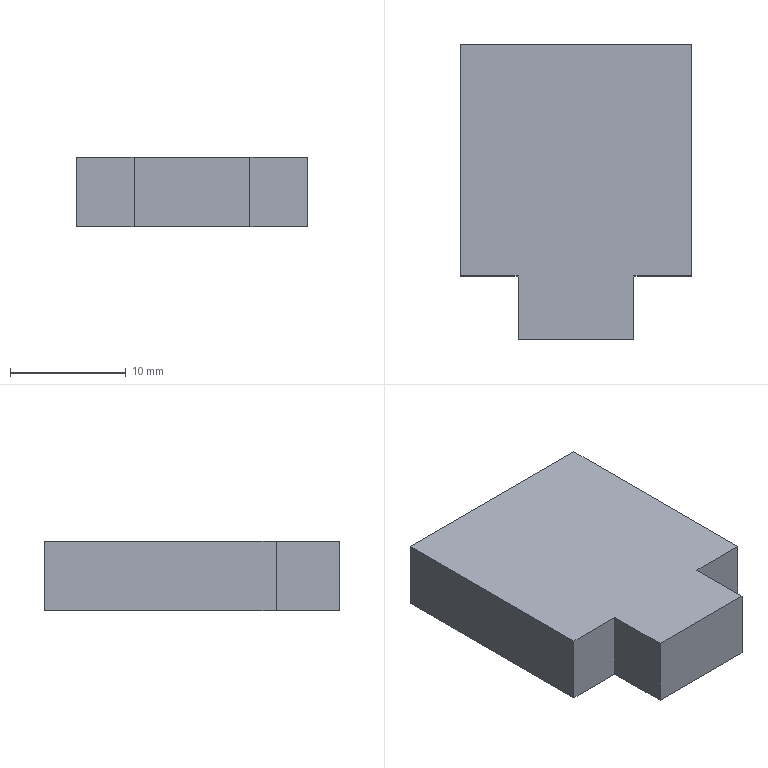Part | SolidWorks | features FlatPattern 1, SMBaseFlange 1, SheetMetal 1 | 1 solid | 10 faces | box 20 x 25.5 x 6 mm | volume 2730 mm3 | plane 10
STEP:
#1=CARTESIAN_POINT('',(50.677,0.,0.));
#2=VERTEX_POINT('',#1);
#3=CARTESIAN_POINT('',(50.677,-5.5,0.));
#4=VERTEX_POINT('',#3);
#5=CARTESIAN_POINT('',(50.677,0.,0.));
#6=DIRECTION('',(0.,-1.,0.));
#7=VECTOR('',#6,1000.);
#8=LINE('',#5,#7);
#9=EDGE_CURVE('',#2,#4,#8,.T.);
#10=ORIENTED_EDGE('',*,*,#9,.T.);
#11=CARTESIAN_POINT('',(50.677,-5.5,6.));
#12=VERTEX_POINT('',#11);
#13=CARTESIAN_POINT('',(50.677,-5.5,6.));
#14=DIRECTION('',(0.,0.,-1.));
#15=VECTOR('',#14,1000.);
#16=LINE('',#13,#15);
#17=EDGE_CURVE('',#12,#4,#16,.T.);
#18=ORIENTED_EDGE('',*,*,#17,.F.);
#19=CARTESIAN_POINT('',(50.677,0.,6.));
#20=VERTEX_POINT('',#19);
#21=CARTESIAN_POINT('',(50.677,0.,6.));
#22=DIRECTION('',(0.,-1.,0.));
#23=VECTOR('',#22,1000.);
#24=LINE('',#21,#23);
#25=EDGE_CURVE('',#20,#12,#24,.T.);
#26=ORIENTED_EDGE('',*,*,#25,.F.);
#27=CARTESIAN_POINT('',(50.677,0.,6.));
#28=DIRECTION('',(0.,0.,-1.));
#29=VECTOR('',#28,1000.);
#30=LINE('',#27,#29);
#31=EDGE_CURVE('',#20,#2,#30,.T.);
#32=ORIENTED_EDGE('',*,*,#31,.T.);
#33=EDGE_LOOP('',(#10,#18,#26,#32));
#34=FACE_OUTER_BOUND('',#33,.T.);
#35=CARTESIAN_POINT('',(50.677,0.,6.));
#36=DIRECTION('',(1.,0.,0.));
#37=DIRECTION('',(0.,0.,-1.));
#38=AXIS2_PLACEMENT_3D('',#35,#36,#37);
#39=PLANE('',#38);
#40=ADVANCED_FACE('',(#34),#39,.F.);
#41=CARTESIAN_POINT('',(60.677,-5.5,0.));
#42=VERTEX_POINT('',#41);
#43=CARTESIAN_POINT('',(50.677,-5.5,0.));
#44=DIRECTION('',(1.,0.,0.));
#45=VECTOR('',#44,1000.);
#46=LINE('',#43,#45);
#47=EDGE_CURVE('',#4,#42,#46,.T.);
#48=ORIENTED_EDGE('',*,*,#47,.T.);
#49=CARTESIAN_POINT('',(60.677,-5.5,6.));
#50=VERTEX_POINT('',#49);
#51=CARTESIAN_POINT('',(60.677,-5.5,6.));
#52=DIRECTION('',(0.,0.,-1.));
#53=VECTOR('',#52,1000.);
#54=LINE('',#51,#53);
#55=EDGE_CURVE('',#50,#42,#54,.T.);
#56=ORIENTED_EDGE('',*,*,#55,.F.);
#57=CARTESIAN_POINT('',(50.677,-5.5,6.));
#58=DIRECTION('',(1.,0.,0.));
#59=VECTOR('',#58,1000.);
#60=LINE('',#57,#59);
#61=EDGE_CURVE('',#12,#50,#60,.T.);
#62=ORIENTED_EDGE('',*,*,#61,.F.);
#63=ORIENTED_EDGE('',*,*,#17,.T.);
#64=EDGE_LOOP('',(#48,#56,#62,#63));
#65=FACE_OUTER_BOUND('',#64,.T.);
#66=CARTESIAN_POINT('',(50.677,-5.5,6.));
#67=DIRECTION('',(0.,1.,0.));
#68=DIRECTION('',(0.,0.,1.));
#69=AXIS2_PLACEMENT_3D('',#66,#67,#68);
#70=PLANE('',#69);
#71=ADVANCED_FACE('',(#65),#70,.F.);
#72=CARTESIAN_POINT('',(60.677,0.,0.));
#73=VERTEX_POINT('',#72);
#74=CARTESIAN_POINT('',(60.677,-5.5,0.));
#75=DIRECTION('',(0.,1.,0.));
#76=VECTOR('',#75,1000.);
#77=LINE('',#74,#76);
#78=EDGE_CURVE('',#42,#73,#77,.T.);
#79=ORIENTED_EDGE('',*,*,#78,.T.);
#80=CARTESIAN_POINT('',(60.677,0.,6.));
#81=VERTEX_POINT('',#80);
#82=CARTESIAN_POINT('',(60.677,0.,6.));
#83=DIRECTION('',(0.,0.,-1.));
#84=VECTOR('',#83,1000.);
#85=LINE('',#82,#84);
#86=EDGE_CURVE('',#81,#73,#85,.T.);
#87=ORIENTED_EDGE('',*,*,#86,.F.);
#88=CARTESIAN_POINT('',(60.677,-5.5,6.));
#89=DIRECTION('',(0.,1.,0.));
#90=VECTOR('',#89,1000.);
#91=LINE('',#88,#90);
#92=EDGE_CURVE('',#50,#81,#91,.T.);
#93=ORIENTED_EDGE('',*,*,#92,.F.);
#94=ORIENTED_EDGE('',*,*,#55,.T.);
#95=EDGE_LOOP('',(#79,#87,#93,#94));
#96=FACE_OUTER_BOUND('',#95,.T.);
#97=CARTESIAN_POINT('',(60.677,-5.5,6.));
#98=DIRECTION('',(-1.,0.,0.));
#99=DIRECTION('',(0.,0.,1.));
#100=AXIS2_PLACEMENT_3D('',#97,#98,#99);
#101=PLANE('',#100);
#102=ADVANCED_FACE('',(#96),#101,.F.);
#103=CARTESIAN_POINT('',(65.677,0.,0.));
#104=VERTEX_POINT('',#103);
#105=CARTESIAN_POINT('',(60.677,0.,0.));
#106=DIRECTION('',(1.,0.,0.));
#107=VECTOR('',#106,1000.);
#108=LINE('',#105,#107);
#109=EDGE_CURVE('',#73,#104,#108,.T.);
#110=ORIENTED_EDGE('',*,*,#109,.T.);
#111=CARTESIAN_POINT('',(65.677,0.,6.));
#112=VERTEX_POINT('',#111);
#113=CARTESIAN_POINT('',(65.677,0.,6.));
#114=DIRECTION('',(0.,0.,-1.));
#115=VECTOR('',#114,1000.);
#116=LINE('',#113,#115);
#117=EDGE_CURVE('',#112,#104,#116,.T.);
#118=ORIENTED_EDGE('',*,*,#117,.F.);
#119=CARTESIAN_POINT('',(60.677,0.,6.));
#120=DIRECTION('',(1.,0.,0.));
#121=VECTOR('',#120,1000.);
#122=LINE('',#119,#121);
#123=EDGE_CURVE('',#81,#112,#122,.T.);
#124=ORIENTED_EDGE('',*,*,#123,.F.);
#125=ORIENTED_EDGE('',*,*,#86,.T.);
#126=EDGE_LOOP('',(#110,#118,#124,#125));
#127=FACE_OUTER_BOUND('',#126,.T.);
#128=CARTESIAN_POINT('',(60.677,0.,6.));
#129=DIRECTION('',(0.,1.,0.));
#130=DIRECTION('',(-1.,0.,0.));
#131=AXIS2_PLACEMENT_3D('',#128,#129,#130);
#132=PLANE('',#131);
#133=ADVANCED_FACE('',(#127),#132,.F.);
#134=CARTESIAN_POINT('',(65.677,20.,0.));
#135=VERTEX_POINT('',#134);
#136=CARTESIAN_POINT('',(65.677,0.,0.));
#137=DIRECTION('',(0.,1.,0.));
#138=VECTOR('',#137,1000.);
#139=LINE('',#136,#138);
#140=EDGE_CURVE('',#104,#135,#139,.T.);
#141=ORIENTED_EDGE('',*,*,#140,.T.);
#142=CARTESIAN_POINT('',(65.677,20.,6.));
#143=VERTEX_POINT('',#142);
#144=CARTESIAN_POINT('',(65.677,20.,6.));
#145=DIRECTION('',(0.,0.,-1.));
#146=VECTOR('',#145,1000.);
#147=LINE('',#144,#146);
#148=EDGE_CURVE('',#143,#135,#147,.T.);
#149=ORIENTED_EDGE('',*,*,#148,.F.);
#150=CARTESIAN_POINT('',(65.677,0.,6.));
#151=DIRECTION('',(0.,1.,0.));
#152=VECTOR('',#151,1000.);
#153=LINE('',#150,#152);
#154=EDGE_CURVE('',#112,#143,#153,.T.);
#155=ORIENTED_EDGE('',*,*,#154,.F.);
#156=ORIENTED_EDGE('',*,*,#117,.T.);
#157=EDGE_LOOP('',(#141,#149,#155,#156));
#158=FACE_OUTER_BOUND('',#157,.T.);
#159=CARTESIAN_POINT('',(65.677,0.,6.));
#160=DIRECTION('',(-1.,0.,0.));
#161=DIRECTION('',(0.,0.,1.));
#162=AXIS2_PLACEMENT_3D('',#159,#160,#161);
#163=PLANE('',#162);
#164=ADVANCED_FACE('',(#158),#163,.F.);
#165=CARTESIAN_POINT('',(45.677,20.,0.));
#166=VERTEX_POINT('',#165);
#167=CARTESIAN_POINT('',(65.677,20.,0.));
#168=DIRECTION('',(-1.,0.,0.));
#169=VECTOR('',#168,1000.);
#170=LINE('',#167,#169);
#171=EDGE_CURVE('',#135,#166,#170,.T.);
#172=ORIENTED_EDGE('',*,*,#171,.T.);
#173=CARTESIAN_POINT('',(45.677,20.,6.));
#174=VERTEX_POINT('',#173);
#175=CARTESIAN_POINT('',(45.677,20.,6.));
#176=DIRECTION('',(0.,0.,-1.));
#177=VECTOR('',#176,1000.);
#178=LINE('',#175,#177);
#179=EDGE_CURVE('',#174,#166,#178,.T.);
#180=ORIENTED_EDGE('',*,*,#179,.F.);
#181=CARTESIAN_POINT('',(65.677,20.,6.));
#182=DIRECTION('',(-1.,0.,0.));
#183=VECTOR('',#182,1000.);
#184=LINE('',#181,#183);
#185=EDGE_CURVE('',#143,#174,#184,.T.);
#186=ORIENTED_EDGE('',*,*,#185,.F.);
#187=ORIENTED_EDGE('',*,*,#148,.T.);
#188=EDGE_LOOP('',(#172,#180,#186,#187));
#189=FACE_OUTER_BOUND('',#188,.T.);
#190=CARTESIAN_POINT('',(65.677,20.,6.));
#191=DIRECTION('',(0.,-1.,0.));
#192=DIRECTION('',(1.,0.,0.));
#193=AXIS2_PLACEMENT_3D('',#190,#191,#192);
#194=PLANE('',#193);
#195=ADVANCED_FACE('',(#189),#194,.F.);
#196=CARTESIAN_POINT('',(45.677,0.,0.));
#197=VERTEX_POINT('',#196);
#198=CARTESIAN_POINT('',(45.677,20.,0.));
#199=DIRECTION('',(0.,-1.,0.));
#200=VECTOR('',#199,1000.);
#201=LINE('',#198,#200);
#202=EDGE_CURVE('',#166,#197,#201,.T.);
#203=ORIENTED_EDGE('',*,*,#202,.T.);
#204=CARTESIAN_POINT('',(45.677,0.,6.));
#205=VERTEX_POINT('',#204);
#206=CARTESIAN_POINT('',(45.677,0.,6.));
#207=DIRECTION('',(0.,0.,-1.));
#208=VECTOR('',#207,1000.);
#209=LINE('',#206,#208);
#210=EDGE_CURVE('',#205,#197,#209,.T.);
#211=ORIENTED_EDGE('',*,*,#210,.F.);
#212=CARTESIAN_POINT('',(45.677,20.,6.));
#213=DIRECTION('',(0.,-1.,0.));
#214=VECTOR('',#213,1000.);
#215=LINE('',#212,#214);
#216=EDGE_CURVE('',#174,#205,#215,.T.);
#217=ORIENTED_EDGE('',*,*,#216,.F.);
#218=ORIENTED_EDGE('',*,*,#179,.T.);
#219=EDGE_LOOP('',(#203,#211,#217,#218));
#220=FACE_OUTER_BOUND('',#219,.T.);
#221=CARTESIAN_POINT('',(45.677,20.,6.));
#222=DIRECTION('',(1.,0.,0.));
#223=DIRECTION('',(0.,0.,-1.));
#224=AXIS2_PLACEMENT_3D('',#221,#222,#223);
#225=PLANE('',#224);
#226=ADVANCED_FACE('',(#220),#225,.F.);
#227=CARTESIAN_POINT('',(45.677,0.,0.));
#228=DIRECTION('',(1.,0.,0.));
#229=VECTOR('',#228,1000.);
#230=LINE('',#227,#229);
#231=EDGE_CURVE('',#197,#2,#230,.T.);
#232=ORIENTED_EDGE('',*,*,#231,.T.);
#233=ORIENTED_EDGE('',*,*,#31,.F.);
#234=CARTESIAN_POINT('',(45.677,0.,6.));
#235=DIRECTION('',(1.,0.,0.));
#236=VECTOR('',#235,1000.);
#237=LINE('',#234,#236);
#238=EDGE_CURVE('',#205,#20,#237,.T.);
#239=ORIENTED_EDGE('',*,*,#238,.F.);
#240=ORIENTED_EDGE('',*,*,#210,.T.);
#241=EDGE_LOOP('',(#232,#233,#239,#240));
#242=FACE_OUTER_BOUND('',#241,.T.);
#243=CARTESIAN_POINT('',(45.677,0.,6.));
#244=DIRECTION('',(0.,1.,0.));
#245=DIRECTION('',(-1.,0.,0.));
#246=AXIS2_PLACEMENT_3D('',#243,#244,#245);
#247=PLANE('',#246);
#248=ADVANCED_FACE('',(#242),#247,.F.);
#249=ORIENTED_EDGE('',*,*,#25,.T.);
#250=ORIENTED_EDGE('',*,*,#61,.T.);
#251=ORIENTED_EDGE('',*,*,#92,.T.);
#252=ORIENTED_EDGE('',*,*,#123,.T.);
#253=ORIENTED_EDGE('',*,*,#154,.T.);
#254=ORIENTED_EDGE('',*,*,#185,.T.);
#255=ORIENTED_EDGE('',*,*,#216,.T.);
#256=ORIENTED_EDGE('',*,*,#238,.T.);
#257=EDGE_LOOP('',(#249,#250,#251,#252,#253,#254,#255,#256));
#258=FACE_OUTER_BOUND('',#257,.T.);
#259=CARTESIAN_POINT('',(0.,0.,6.));
#260=DIRECTION('',(0.,0.,1.));
#261=DIRECTION('',(1.,0.,0.));
#262=AXIS2_PLACEMENT_3D('',#259,#260,#261);
#263=PLANE('',#262);
#264=ADVANCED_FACE('',(#258),#263,.T.);
#265=ORIENTED_EDGE('',*,*,#9,.F.);
#266=ORIENTED_EDGE('',*,*,#231,.F.);
#267=ORIENTED_EDGE('',*,*,#202,.F.);
#268=ORIENTED_EDGE('',*,*,#171,.F.);
#269=ORIENTED_EDGE('',*,*,#140,.F.);
#270=ORIENTED_EDGE('',*,*,#109,.F.);
#271=ORIENTED_EDGE('',*,*,#78,.F.);
#272=ORIENTED_EDGE('',*,*,#47,.F.);
#273=EDGE_LOOP('',(#265,#266,#267,#268,#269,#270,#271,#272));
#274=FACE_OUTER_BOUND('',#273,.T.);
#275=CARTESIAN_POINT('',(0.,0.,0.));
#276=DIRECTION('',(0.,0.,1.));
#277=DIRECTION('',(1.,0.,0.));
#278=AXIS2_PLACEMENT_3D('',#275,#276,#277);
#279=PLANE('',#278);
#280=ADVANCED_FACE('',(#274),#279,.F.);
#281=CLOSED_SHELL('',(#40,#71,#102,#133,#164,#195,#226,#248,#264,#280));
#282=MANIFOLD_SOLID_BREP('',#281);
#283=CARTESIAN_POINT('',(0.,0.,0.));
#284=DIRECTION('',(0.,0.,1.));
#285=DIRECTION('',(1.,0.,0.));
#286=AXIS2_PLACEMENT_3D('',#283,#284,#285);
#287=(LENGTH_UNIT()NAMED_UNIT(*)SI_UNIT(.MILLI.,.METRE.));
#288=UNCERTAINTY_MEASURE_WITH_UNIT(LENGTH_MEASURE(0.00001),#287,'','');
#289=(NAMED_UNIT(*)PLANE_ANGLE_UNIT()SI_UNIT($,.RADIAN.));
#290=(NAMED_UNIT(*)SI_UNIT($,.STERADIAN.)SOLID_ANGLE_UNIT());
#291=(GEOMETRIC_REPRESENTATION_CONTEXT(3)GLOBAL_UNCERTAINTY_ASSIGNED_CONTEXT((#288))GLOBAL_UNIT_ASSIGNED_CONTEXT((#287,#289,#290))REPRESENTATION_CONTEXT('',''));
#292=ADVANCED_BREP_SHAPE_REPRESENTATION('',(#282,#286),#291);